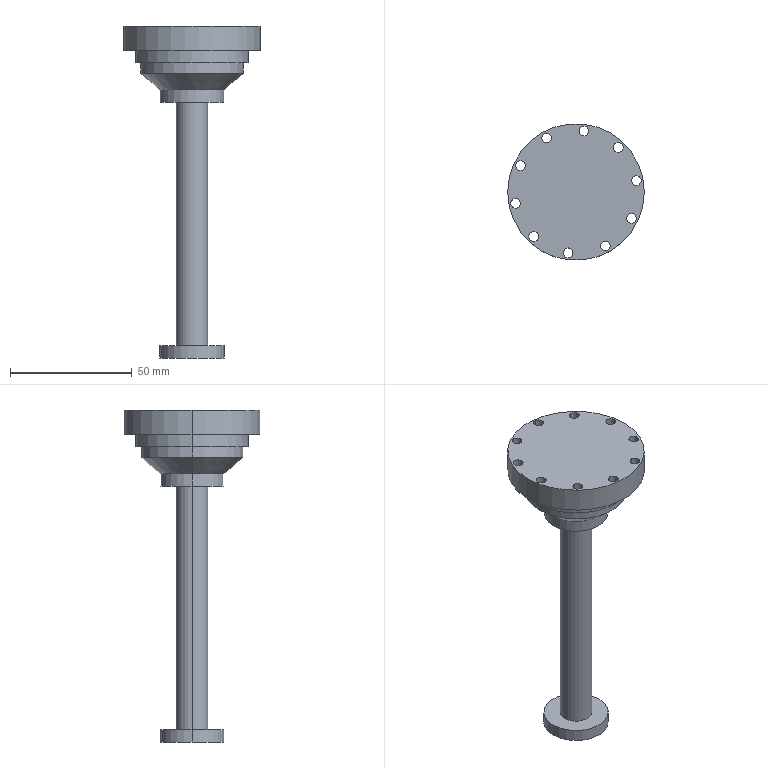Part | SolidWorks | features CirPattern 1, Cut 1, ICE 1, RevCut 1, Revolution 1 | 1 solid | 40 faces | box 56 x 56 x 136.215 mm | volume 62854 mm3 | cylinder 26 | cone 8 | plane 6 | commonest cylinder face diameters 4 x20 13.058 x2 42 x2 56 x2
STEP:
#1=CARTESIAN_POINT('',(-0.7415,66.642,15.));
#2=VERTEX_POINT('',#1);
#3=CARTESIAN_POINT('',(-4.741,66.642,15.));
#4=VERTEX_POINT('',#3);
#5=CARTESIAN_POINT('',(-2.741,66.642,15.));
#6=DIRECTION('',(0.,0.,-1.));
#7=DIRECTION('',(-0.809,0.5878,0.));
#8=AXIS2_PLACEMENT_3D('',#5,#6,#7);
#9=CIRCLE('',#8,2.);
#10=EDGE_CURVE('',#2,#4,#9,.T.);
#11=ORIENTED_EDGE('',*,*,#10,.F.);
#12=CARTESIAN_POINT('',(-0.7415,66.642,5.));
#13=VERTEX_POINT('',#12);
#14=CARTESIAN_POINT('',(-0.7415,66.642,15.));
#15=DIRECTION('',(0.,0.,-1.));
#16=VECTOR('',#15,1000.);
#17=LINE('',#14,#16);
#18=EDGE_CURVE('',#2,#13,#17,.T.);
#19=ORIENTED_EDGE('',*,*,#18,.T.);
#20=CARTESIAN_POINT('',(-4.741,66.642,5.));
#21=VERTEX_POINT('',#20);
#22=CARTESIAN_POINT('',(-2.741,66.642,5.));
#23=DIRECTION('',(0.,0.,-1.));
#24=DIRECTION('',(-0.809,0.5878,0.));
#25=AXIS2_PLACEMENT_3D('',#22,#23,#24);
#26=CIRCLE('',#25,2.);
#27=EDGE_CURVE('',#13,#21,#26,.T.);
#28=ORIENTED_EDGE('',*,*,#27,.T.);
#29=CARTESIAN_POINT('',(-4.741,66.642,15.));
#30=DIRECTION('',(0.,0.,-1.));
#31=VECTOR('',#30,1000.);
#32=LINE('',#29,#31);
#33=EDGE_CURVE('',#4,#21,#32,.T.);
#34=ORIENTED_EDGE('',*,*,#33,.F.);
#35=EDGE_LOOP('',(#11,#19,#28,#34));
#36=FACE_OUTER_BOUND('',#35,.T.);
#37=CARTESIAN_POINT('',(-2.741,66.642,15.));
#38=DIRECTION('',(0.,0.,-1.));
#39=DIRECTION('',(-1.,0.,0.));
#40=AXIS2_PLACEMENT_3D('',#37,#38,#39);
#41=CYLINDRICAL_SURFACE('',#40,2.);
#42=ADVANCED_FACE('',(#36),#41,.F.);
#43=CARTESIAN_POINT('',(7.956,75.944,15.));
#44=VERTEX_POINT('',#43);
#45=CARTESIAN_POINT('',(7.956,79.944,15.));
#46=VERTEX_POINT('',#45);
#47=CARTESIAN_POINT('',(7.956,77.944,15.));
#48=DIRECTION('',(0.,0.,-1.));
#49=DIRECTION('',(-0.309,0.9511,0.));
#50=AXIS2_PLACEMENT_3D('',#47,#48,#49);
#51=CIRCLE('',#50,2.);
#52=EDGE_CURVE('',#44,#46,#51,.T.);
#53=ORIENTED_EDGE('',*,*,#52,.F.);
#54=CARTESIAN_POINT('',(7.956,75.944,5.));
#55=VERTEX_POINT('',#54);
#56=CARTESIAN_POINT('',(7.956,75.944,15.));
#57=DIRECTION('',(0.,0.,-1.));
#58=VECTOR('',#57,1000.);
#59=LINE('',#56,#58);
#60=EDGE_CURVE('',#44,#55,#59,.T.);
#61=ORIENTED_EDGE('',*,*,#60,.T.);
#62=CARTESIAN_POINT('',(7.956,79.944,5.));
#63=VERTEX_POINT('',#62);
#64=CARTESIAN_POINT('',(7.956,77.944,5.));
#65=DIRECTION('',(0.,0.,-1.));
#66=DIRECTION('',(-0.309,0.9511,0.));
#67=AXIS2_PLACEMENT_3D('',#64,#65,#66);
#68=CIRCLE('',#67,2.);
#69=EDGE_CURVE('',#55,#63,#68,.T.);
#70=ORIENTED_EDGE('',*,*,#69,.T.);
#71=CARTESIAN_POINT('',(7.956,79.944,15.));
#72=DIRECTION('',(0.,0.,-1.));
#73=VECTOR('',#72,1000.);
#74=LINE('',#71,#73);
#75=EDGE_CURVE('',#46,#63,#74,.T.);
#76=ORIENTED_EDGE('',*,*,#75,.F.);
#77=EDGE_LOOP('',(#53,#61,#70,#76));
#78=FACE_OUTER_BOUND('',#77,.T.);
#79=CARTESIAN_POINT('',(7.956,77.944,15.));
#80=DIRECTION('',(0.,0.,-1.));
#81=DIRECTION('',(0.,1.,0.));
#82=AXIS2_PLACEMENT_3D('',#79,#80,#81);
#83=CYLINDRICAL_SURFACE('',#82,2.);
#84=ADVANCED_FACE('',(#78),#83,.F.);
#85=CARTESIAN_POINT('',(23.255,78.8,15.));
#86=VERTEX_POINT('',#85);
#87=CARTESIAN_POINT('',(23.255,82.8,15.));
#88=VERTEX_POINT('',#87);
#89=CARTESIAN_POINT('',(23.255,80.8,15.));
#90=DIRECTION('',(0.,0.,-1.));
#91=DIRECTION('',(0.309,0.9511,0.));
#92=AXIS2_PLACEMENT_3D('',#89,#90,#91);
#93=CIRCLE('',#92,2.);
#94=EDGE_CURVE('',#86,#88,#93,.T.);
#95=ORIENTED_EDGE('',*,*,#94,.F.);
#96=CARTESIAN_POINT('',(23.255,78.8,5.));
#97=VERTEX_POINT('',#96);
#98=CARTESIAN_POINT('',(23.255,78.8,15.));
#99=DIRECTION('',(0.,0.,-1.));
#100=VECTOR('',#99,1000.);
#101=LINE('',#98,#100);
#102=EDGE_CURVE('',#86,#97,#101,.T.);
#103=ORIENTED_EDGE('',*,*,#102,.T.);
#104=CARTESIAN_POINT('',(23.255,82.8,5.));
#105=VERTEX_POINT('',#104);
#106=CARTESIAN_POINT('',(23.255,80.8,5.));
#107=DIRECTION('',(0.,0.,-1.));
#108=DIRECTION('',(0.309,0.9511,0.));
#109=AXIS2_PLACEMENT_3D('',#106,#107,#108);
#110=CIRCLE('',#109,2.);
#111=EDGE_CURVE('',#97,#105,#110,.T.);
#112=ORIENTED_EDGE('',*,*,#111,.T.);
#113=CARTESIAN_POINT('',(23.255,82.8,15.));
#114=DIRECTION('',(0.,0.,-1.));
#115=VECTOR('',#114,1000.);
#116=LINE('',#113,#115);
#117=EDGE_CURVE('',#88,#105,#116,.T.);
#118=ORIENTED_EDGE('',*,*,#117,.F.);
#119=EDGE_LOOP('',(#95,#103,#112,#118));
#120=FACE_OUTER_BOUND('',#119,.T.);
#121=CARTESIAN_POINT('',(23.255,80.8,15.));
#122=DIRECTION('',(0.,0.,-1.));
#123=DIRECTION('',(0.,1.,0.));
#124=AXIS2_PLACEMENT_3D('',#121,#122,#123);
#125=CYLINDRICAL_SURFACE('',#124,2.);
#126=ADVANCED_FACE('',(#120),#125,.F.);
#127=CARTESIAN_POINT('',(37.31,72.118,15.));
#128=VERTEX_POINT('',#127);
#129=CARTESIAN_POINT('',(37.31,76.118,15.));
#130=VERTEX_POINT('',#129);
#131=CARTESIAN_POINT('',(37.31,74.118,15.));
#132=DIRECTION('',(0.,0.,-1.));
#133=DIRECTION('',(0.809,0.5878,0.));
#134=AXIS2_PLACEMENT_3D('',#131,#132,#133);
#135=CIRCLE('',#134,2.);
#136=EDGE_CURVE('',#128,#130,#135,.T.);
#137=ORIENTED_EDGE('',*,*,#136,.F.);
#138=CARTESIAN_POINT('',(37.31,72.118,5.));
#139=VERTEX_POINT('',#138);
#140=CARTESIAN_POINT('',(37.31,72.118,15.));
#141=DIRECTION('',(0.,0.,-1.));
#142=VECTOR('',#141,1000.);
#143=LINE('',#140,#142);
#144=EDGE_CURVE('',#128,#139,#143,.T.);
#145=ORIENTED_EDGE('',*,*,#144,.T.);
#146=CARTESIAN_POINT('',(37.31,76.118,5.));
#147=VERTEX_POINT('',#146);
#148=CARTESIAN_POINT('',(37.31,74.118,5.));
#149=DIRECTION('',(0.,0.,-1.));
#150=DIRECTION('',(0.809,0.5878,0.));
#151=AXIS2_PLACEMENT_3D('',#148,#149,#150);
#152=CIRCLE('',#151,2.);
#153=EDGE_CURVE('',#139,#147,#152,.T.);
#154=ORIENTED_EDGE('',*,*,#153,.T.);
#155=CARTESIAN_POINT('',(37.31,76.118,15.));
#156=DIRECTION('',(0.,0.,-1.));
#157=VECTOR('',#156,1000.);
#158=LINE('',#155,#157);
#159=EDGE_CURVE('',#130,#147,#158,.T.);
#160=ORIENTED_EDGE('',*,*,#159,.F.);
#161=EDGE_LOOP('',(#137,#145,#154,#160));
#162=FACE_OUTER_BOUND('',#161,.T.);
#163=CARTESIAN_POINT('',(37.31,74.118,15.));
#164=DIRECTION('',(0.,0.,-1.));
#165=DIRECTION('',(0.,1.,0.));
#166=AXIS2_PLACEMENT_3D('',#163,#164,#165);
#167=CYLINDRICAL_SURFACE('',#166,2.);
#168=ADVANCED_FACE('',(#162),#167,.F.);
#169=CARTESIAN_POINT('',(46.753,60.451,15.));
#170=VERTEX_POINT('',#169);
#171=CARTESIAN_POINT('',(42.753,60.451,15.));
#172=VERTEX_POINT('',#171);
#173=CARTESIAN_POINT('',(44.753,60.451,15.));
#174=DIRECTION('',(0.,0.,-1.));
#175=DIRECTION('',(1.,0.,0.));
#176=AXIS2_PLACEMENT_3D('',#173,#174,#175);
#177=CIRCLE('',#176,2.);
#178=EDGE_CURVE('',#170,#172,#177,.T.);
#179=ORIENTED_EDGE('',*,*,#178,.F.);
#180=CARTESIAN_POINT('',(46.753,60.451,5.));
#181=VERTEX_POINT('',#180);
#182=CARTESIAN_POINT('',(46.753,60.451,15.));
#183=DIRECTION('',(0.,0.,-1.));
#184=VECTOR('',#183,1000.);
#185=LINE('',#182,#184);
#186=EDGE_CURVE('',#170,#181,#185,.T.);
#187=ORIENTED_EDGE('',*,*,#186,.T.);
#188=CARTESIAN_POINT('',(42.753,60.451,5.));
#189=VERTEX_POINT('',#188);
#190=CARTESIAN_POINT('',(44.753,60.451,5.));
#191=DIRECTION('',(0.,0.,-1.));
#192=DIRECTION('',(1.,0.,0.));
#193=AXIS2_PLACEMENT_3D('',#190,#191,#192);
#194=CIRCLE('',#193,2.);
#195=EDGE_CURVE('',#181,#189,#194,.T.);
#196=ORIENTED_EDGE('',*,*,#195,.T.);
#197=CARTESIAN_POINT('',(42.753,60.451,15.));
#198=DIRECTION('',(0.,0.,-1.));
#199=VECTOR('',#198,1000.);
#200=LINE('',#197,#199);
#201=EDGE_CURVE('',#172,#189,#200,.T.);
#202=ORIENTED_EDGE('',*,*,#201,.F.);
#203=EDGE_LOOP('',(#179,#187,#196,#202));
#204=FACE_OUTER_BOUND('',#203,.T.);
#205=CARTESIAN_POINT('',(44.753,60.451,15.));
#206=DIRECTION('',(0.,0.,-1.));
#207=DIRECTION('',(-1.,0.,0.));
#208=AXIS2_PLACEMENT_3D('',#205,#206,#207);
#209=CYLINDRICAL_SURFACE('',#208,2.);
#210=ADVANCED_FACE('',(#204),#209,.F.);
#211=CARTESIAN_POINT('',(44.741,45.019,15.));
#212=VERTEX_POINT('',#211);
#213=CARTESIAN_POINT('',(40.741,45.019,15.));
#214=VERTEX_POINT('',#213);
#215=CARTESIAN_POINT('',(42.741,45.019,15.));
#216=DIRECTION('',(0.,0.,-1.));
#217=DIRECTION('',(0.809,-0.5878,0.));
#218=AXIS2_PLACEMENT_3D('',#215,#216,#217);
#219=CIRCLE('',#218,2.);
#220=EDGE_CURVE('',#212,#214,#219,.T.);
#221=ORIENTED_EDGE('',*,*,#220,.F.);
#222=CARTESIAN_POINT('',(44.741,45.019,5.));
#223=VERTEX_POINT('',#222);
#224=CARTESIAN_POINT('',(44.741,45.019,15.));
#225=DIRECTION('',(0.,0.,-1.));
#226=VECTOR('',#225,1000.);
#227=LINE('',#224,#226);
#228=EDGE_CURVE('',#212,#223,#227,.T.);
#229=ORIENTED_EDGE('',*,*,#228,.T.);
#230=CARTESIAN_POINT('',(40.741,45.019,5.));
#231=VERTEX_POINT('',#230);
#232=CARTESIAN_POINT('',(42.741,45.019,5.));
#233=DIRECTION('',(0.,0.,-1.));
#234=DIRECTION('',(0.809,-0.5878,0.));
#235=AXIS2_PLACEMENT_3D('',#232,#233,#234);
#236=CIRCLE('',#235,2.);
#237=EDGE_CURVE('',#223,#231,#236,.T.);
#238=ORIENTED_EDGE('',*,*,#237,.T.);
#239=CARTESIAN_POINT('',(40.741,45.019,15.));
#240=DIRECTION('',(0.,0.,-1.));
#241=VECTOR('',#240,1000.);
#242=LINE('',#239,#241);
#243=EDGE_CURVE('',#214,#231,#242,.T.);
#244=ORIENTED_EDGE('',*,*,#243,.F.);
#245=EDGE_LOOP('',(#221,#229,#238,#244));
#246=FACE_OUTER_BOUND('',#245,.T.);
#247=CARTESIAN_POINT('',(42.741,45.019,15.));
#248=DIRECTION('',(0.,0.,-1.));
#249=DIRECTION('',(-1.,0.,0.));
#250=AXIS2_PLACEMENT_3D('',#247,#248,#249);
#251=CYLINDRICAL_SURFACE('',#250,2.);
#252=ADVANCED_FACE('',(#246),#251,.F.);
#253=CARTESIAN_POINT('',(32.044,31.717,15.));
#254=VERTEX_POINT('',#253);
#255=CARTESIAN_POINT('',(32.044,35.717,15.));
#256=VERTEX_POINT('',#255);
#257=CARTESIAN_POINT('',(32.044,33.717,15.));
#258=DIRECTION('',(0.,0.,-1.));
#259=DIRECTION('',(0.309,-0.9511,0.));
#260=AXIS2_PLACEMENT_3D('',#257,#258,#259);
#261=CIRCLE('',#260,2.);
#262=EDGE_CURVE('',#254,#256,#261,.T.);
#263=ORIENTED_EDGE('',*,*,#262,.F.);
#264=CARTESIAN_POINT('',(32.044,31.717,5.));
#265=VERTEX_POINT('',#264);
#266=CARTESIAN_POINT('',(32.044,31.717,15.));
#267=DIRECTION('',(0.,0.,-1.));
#268=VECTOR('',#267,1000.);
#269=LINE('',#266,#268);
#270=EDGE_CURVE('',#254,#265,#269,.T.);
#271=ORIENTED_EDGE('',*,*,#270,.T.);
#272=CARTESIAN_POINT('',(32.044,35.717,5.));
#273=VERTEX_POINT('',#272);
#274=CARTESIAN_POINT('',(32.044,33.717,5.));
#275=DIRECTION('',(0.,0.,-1.));
#276=DIRECTION('',(0.309,-0.9511,0.));
#277=AXIS2_PLACEMENT_3D('',#274,#275,#276);
#278=CIRCLE('',#277,2.);
#279=EDGE_CURVE('',#265,#273,#278,.T.);
#280=ORIENTED_EDGE('',*,*,#279,.T.);
#281=CARTESIAN_POINT('',(32.044,35.717,15.));
#282=DIRECTION('',(0.,0.,-1.));
#283=VECTOR('',#282,1000.);
#284=LINE('',#281,#283);
#285=EDGE_CURVE('',#256,#273,#284,.T.);
#286=ORIENTED_EDGE('',*,*,#285,.F.);
#287=EDGE_LOOP('',(#263,#271,#280,#286));
#288=FACE_OUTER_BOUND('',#287,.T.);
#289=CARTESIAN_POINT('',(32.044,33.717,15.));
#290=DIRECTION('',(0.,0.,-1.));
#291=DIRECTION('',(0.,1.,0.));
#292=AXIS2_PLACEMENT_3D('',#289,#290,#291);
#293=CYLINDRICAL_SURFACE('',#292,2.);
#294=ADVANCED_FACE('',(#288),#293,.F.);
#295=CARTESIAN_POINT('',(16.745,28.861,15.));
#296=VERTEX_POINT('',#295);
#297=CARTESIAN_POINT('',(16.745,32.861,15.));
#298=VERTEX_POINT('',#297);
#299=CARTESIAN_POINT('',(16.745,30.861,15.));
#300=DIRECTION('',(0.,0.,-1.));
#301=DIRECTION('',(-0.309,-0.9511,0.));
#302=AXIS2_PLACEMENT_3D('',#299,#300,#301);
#303=CIRCLE('',#302,2.);
#304=EDGE_CURVE('',#296,#298,#303,.T.);
#305=ORIENTED_EDGE('',*,*,#304,.F.);
#306=CARTESIAN_POINT('',(16.745,28.861,5.));
#307=VERTEX_POINT('',#306);
#308=CARTESIAN_POINT('',(16.745,28.861,15.));
#309=DIRECTION('',(0.,0.,-1.));
#310=VECTOR('',#309,1000.);
#311=LINE('',#308,#310);
#312=EDGE_CURVE('',#296,#307,#311,.T.);
#313=ORIENTED_EDGE('',*,*,#312,.T.);
#314=CARTESIAN_POINT('',(16.745,32.861,5.));
#315=VERTEX_POINT('',#314);
#316=CARTESIAN_POINT('',(16.745,30.861,5.));
#317=DIRECTION('',(0.,0.,-1.));
#318=DIRECTION('',(-0.309,-0.9511,0.));
#319=AXIS2_PLACEMENT_3D('',#316,#317,#318);
#320=CIRCLE('',#319,2.);
#321=EDGE_CURVE('',#307,#315,#320,.T.);
#322=ORIENTED_EDGE('',*,*,#321,.T.);
#323=CARTESIAN_POINT('',(16.745,32.861,15.));
#324=DIRECTION('',(0.,0.,-1.));
#325=VECTOR('',#324,1000.);
#326=LINE('',#323,#325);
#327=EDGE_CURVE('',#298,#315,#326,.T.);
#328=ORIENTED_EDGE('',*,*,#327,.F.);
#329=EDGE_LOOP('',(#305,#313,#322,#328));
#330=FACE_OUTER_BOUND('',#329,.T.);
#331=CARTESIAN_POINT('',(16.745,30.861,15.));
#332=DIRECTION('',(0.,0.,-1.));
#333=DIRECTION('',(0.,1.,0.));
#334=AXIS2_PLACEMENT_3D('',#331,#332,#333);
#335=CYLINDRICAL_SURFACE('',#334,2.);
#336=ADVANCED_FACE('',(#330),#335,.F.);
#337=CARTESIAN_POINT('',(2.69,35.543,15.));
#338=VERTEX_POINT('',#337);
#339=CARTESIAN_POINT('',(2.69,39.543,15.));
#340=VERTEX_POINT('',#339);
#341=CARTESIAN_POINT('',(2.69,37.543,15.));
#342=DIRECTION('',(0.,0.,-1.));
#343=DIRECTION('',(-0.809,-0.5878,0.));
#344=AXIS2_PLACEMENT_3D('',#341,#342,#343);
#345=CIRCLE('',#344,2.);
#346=EDGE_CURVE('',#338,#340,#345,.T.);
#347=ORIENTED_EDGE('',*,*,#346,.F.);
#348=CARTESIAN_POINT('',(2.69,35.543,5.));
#349=VERTEX_POINT('',#348);
#350=CARTESIAN_POINT('',(2.69,35.543,15.));
#351=DIRECTION('',(0.,0.,-1.));
#352=VECTOR('',#351,1000.);
#353=LINE('',#350,#352);
#354=EDGE_CURVE('',#338,#349,#353,.T.);
#355=ORIENTED_EDGE('',*,*,#354,.T.);
#356=CARTESIAN_POINT('',(2.69,39.543,5.));
#357=VERTEX_POINT('',#356);
#358=CARTESIAN_POINT('',(2.69,37.543,5.));
#359=DIRECTION('',(0.,0.,-1.));
#360=DIRECTION('',(-0.809,-0.5878,0.));
#361=AXIS2_PLACEMENT_3D('',#358,#359,#360);
#362=CIRCLE('',#361,2.);
#363=EDGE_CURVE('',#349,#357,#362,.T.);
#364=ORIENTED_EDGE('',*,*,#363,.T.);
#365=CARTESIAN_POINT('',(2.69,39.543,15.));
#366=DIRECTION('',(0.,0.,-1.));
#367=VECTOR('',#366,1000.);
#368=LINE('',#365,#367);
#369=EDGE_CURVE('',#340,#357,#368,.T.);
#370=ORIENTED_EDGE('',*,*,#369,.F.);
#371=EDGE_LOOP('',(#347,#355,#364,#370));
#372=FACE_OUTER_BOUND('',#371,.T.);
#373=CARTESIAN_POINT('',(2.69,37.543,15.));
#374=DIRECTION('',(0.,0.,-1.));
#375=DIRECTION('',(0.,1.,0.));
#376=AXIS2_PLACEMENT_3D('',#373,#374,#375);
#377=CYLINDRICAL_SURFACE('',#376,2.);
#378=ADVANCED_FACE('',(#372),#377,.F.);
#379=CARTESIAN_POINT('',(-2.753,51.21,15.));
#380=VERTEX_POINT('',#379);
#381=CARTESIAN_POINT('',(-6.753,51.21,15.));
#382=VERTEX_POINT('',#381);
#383=CARTESIAN_POINT('',(-4.753,51.21,15.));
#384=DIRECTION('',(0.,0.,-1.));
#385=DIRECTION('',(-1.,0.,0.));
#386=AXIS2_PLACEMENT_3D('',#383,#384,#385);
#387=CIRCLE('',#386,2.);
#388=EDGE_CURVE('',#380,#382,#387,.T.);
#389=ORIENTED_EDGE('',*,*,#388,.F.);
#390=CARTESIAN_POINT('',(-2.753,51.21,5.));
#391=VERTEX_POINT('',#390);
#392=CARTESIAN_POINT('',(-2.753,51.21,15.));
#393=DIRECTION('',(0.,0.,-1.));
#394=VECTOR('',#393,1000.);
#395=LINE('',#392,#394);
#396=EDGE_CURVE('',#380,#391,#395,.T.);
#397=ORIENTED_EDGE('',*,*,#396,.T.);
#398=CARTESIAN_POINT('',(-6.753,51.21,5.));
#399=VERTEX_POINT('',#398);
#400=CARTESIAN_POINT('',(-4.753,51.21,5.));
#401=DIRECTION('',(0.,0.,-1.));
#402=DIRECTION('',(-1.,0.,0.));
#403=AXIS2_PLACEMENT_3D('',#400,#401,#402);
#404=CIRCLE('',#403,2.);
#405=EDGE_CURVE('',#391,#399,#404,.T.);
#406=ORIENTED_EDGE('',*,*,#405,.T.);
#407=CARTESIAN_POINT('',(-6.753,51.21,15.));
#408=DIRECTION('',(0.,0.,-1.));
#409=VECTOR('',#408,1000.);
#410=LINE('',#407,#409);
#411=EDGE_CURVE('',#382,#399,#410,.T.);
#412=ORIENTED_EDGE('',*,*,#411,.F.);
#413=EDGE_LOOP('',(#389,#397,#406,#412));
#414=FACE_OUTER_BOUND('',#413,.T.);
#415=CARTESIAN_POINT('',(-4.753,51.21,15.));
#416=DIRECTION('',(0.,0.,-1.));
#417=DIRECTION('',(-1.,0.,0.));
#418=AXIS2_PLACEMENT_3D('',#415,#416,#417);
#419=CYLINDRICAL_SURFACE('',#418,2.);
#420=ADVANCED_FACE('',(#414),#419,.F.);
#421=CARTESIAN_POINT('',(-8.,55.831,5.));
#422=VERTEX_POINT('',#421);
#423=CARTESIAN_POINT('',(48.,55.831,5.));
#424=VERTEX_POINT('',#423);
#425=CARTESIAN_POINT('',(20.,55.831,5.));
#426=DIRECTION('',(0.,0.,-1.));
#427=DIRECTION('',(-1.,0.,0.));
#428=AXIS2_PLACEMENT_3D('',#425,#426,#427);
#429=CIRCLE('',#428,28.);
#430=EDGE_CURVE('',#422,#424,#429,.T.);
#431=ORIENTED_EDGE('',*,*,#430,.F.);
#432=CARTESIAN_POINT('',(-8.,55.831,15.));
#433=VERTEX_POINT('',#432);
#434=CARTESIAN_POINT('',(-8.,55.831,5.));
#435=DIRECTION('',(0.,0.,1.));
#436=VECTOR('',#435,1000.);
#437=LINE('',#434,#436);
#438=EDGE_CURVE('',#422,#433,#437,.T.);
#439=ORIENTED_EDGE('',*,*,#438,.T.);
#440=CARTESIAN_POINT('',(48.,55.831,15.));
#441=VERTEX_POINT('',#440);
#442=CARTESIAN_POINT('',(20.,55.831,15.));
#443=DIRECTION('',(0.,0.,-1.));
#444=DIRECTION('',(-1.,0.,0.));
#445=AXIS2_PLACEMENT_3D('',#442,#443,#444);
#446=CIRCLE('',#445,28.);
#447=EDGE_CURVE('',#433,#441,#446,.T.);
#448=ORIENTED_EDGE('',*,*,#447,.T.);
#449=CARTESIAN_POINT('',(48.,55.831,5.));
#450=DIRECTION('',(0.,0.,1.));
#451=VECTOR('',#450,1000.);
#452=LINE('',#449,#451);
#453=EDGE_CURVE('',#424,#441,#452,.T.);
#454=ORIENTED_EDGE('',*,*,#453,.F.);
#455=EDGE_LOOP('',(#431,#439,#448,#454));
#456=FACE_OUTER_BOUND('',#455,.T.);
#457=CARTESIAN_POINT('',(20.,55.831,5.));
#458=DIRECTION('',(0.,0.,1.));
#459=DIRECTION('',(1.,0.,0.));
#460=AXIS2_PLACEMENT_3D('',#457,#458,#459);
#461=CYLINDRICAL_SURFACE('',#460,28.);
#462=ADVANCED_FACE('',(#456),#461,.T.);
#463=CARTESIAN_POINT('',(6.805,55.831,-116.215));
#464=VERTEX_POINT('',#463);
#465=CARTESIAN_POINT('',(33.195,55.831,-116.215));
#466=VERTEX_POINT('',#465);
#467=CARTESIAN_POINT('',(20.,55.831,-116.215));
#468=DIRECTION('',(0.,0.,-1.));
#469=DIRECTION('',(1.,0.,0.));
#470=AXIS2_PLACEMENT_3D('',#467,#468,#469);
#471=CIRCLE('',#470,13.195);
#472=EDGE_CURVE('',#464,#466,#471,.T.);
#473=ORIENTED_EDGE('',*,*,#472,.T.);
#474=CARTESIAN_POINT('',(33.204,55.831,-121.215));
#475=VERTEX_POINT('',#474);
#476=CARTESIAN_POINT('',(33.,55.831,-11.215));
#477=DIRECTION('',(0.001855,0.,-1.));
#478=VECTOR('',#477,1000.);
#479=LINE('',#476,#478);
#480=EDGE_CURVE('',#466,#475,#479,.T.);
#481=ORIENTED_EDGE('',*,*,#480,.T.);
#482=CARTESIAN_POINT('',(6.796,55.831,-121.215));
#483=VERTEX_POINT('',#482);
#484=CARTESIAN_POINT('',(20.,55.831,-121.215));
#485=DIRECTION('',(0.,0.,1.));
#486=DIRECTION('',(1.,0.,0.));
#487=AXIS2_PLACEMENT_3D('',#484,#485,#486);
#488=CIRCLE('',#487,13.204);
#489=EDGE_CURVE('',#475,#483,#488,.T.);
#490=ORIENTED_EDGE('',*,*,#489,.T.);
#491=CARTESIAN_POINT('',(7.,55.831,-11.215));
#492=DIRECTION('',(-0.001855,0.,-1.));
#493=VECTOR('',#492,1000.);
#494=LINE('',#491,#493);
#495=EDGE_CURVE('',#464,#483,#494,.T.);
#496=ORIENTED_EDGE('',*,*,#495,.F.);
#497=EDGE_LOOP('',(#473,#481,#490,#496));
#498=FACE_OUTER_BOUND('',#497,.T.);
#499=CARTESIAN_POINT('',(20.,55.831,-11.215));
#500=DIRECTION('',(0.,0.,-1.));
#501=DIRECTION('',(-1.,0.,0.));
#502=AXIS2_PLACEMENT_3D('',#499,#500,#501);
#503=CONICAL_SURFACE('',#502,13.,0.001855);
#504=ADVANCED_FACE('',(#498),#503,.T.);
#505=CARTESIAN_POINT('',(26.529,55.831,-116.215));
#506=VERTEX_POINT('',#505);
#507=CARTESIAN_POINT('',(13.471,55.831,-116.215));
#508=VERTEX_POINT('',#507);
#509=CARTESIAN_POINT('',(20.,55.831,-116.215));
#510=DIRECTION('',(0.,0.,1.));
#511=DIRECTION('',(1.,0.,0.));
#512=AXIS2_PLACEMENT_3D('',#509,#510,#511);
#513=CIRCLE('',#512,6.529);
#514=EDGE_CURVE('',#506,#508,#513,.T.);
#515=ORIENTED_EDGE('',*,*,#514,.T.);
#516=CARTESIAN_POINT('',(13.471,55.831,-16.215));
#517=VERTEX_POINT('',#516);
#518=CARTESIAN_POINT('',(13.471,55.831,-11.215));
#519=DIRECTION('',(0.,0.,1.));
#520=VECTOR('',#519,1000.);
#521=LINE('',#518,#520);
#522=EDGE_CURVE('',#508,#517,#521,.T.);
#523=ORIENTED_EDGE('',*,*,#522,.T.);
#524=CARTESIAN_POINT('',(26.529,55.831,-16.215));
#525=VERTEX_POINT('',#524);
#526=CARTESIAN_POINT('',(20.,55.831,-16.215));
#527=DIRECTION('',(0.,0.,1.));
#528=DIRECTION('',(1.,0.,0.));
#529=AXIS2_PLACEMENT_3D('',#526,#527,#528);
#530=CIRCLE('',#529,6.529);
#531=EDGE_CURVE('',#525,#517,#530,.T.);
#532=ORIENTED_EDGE('',*,*,#531,.F.);
#533=CARTESIAN_POINT('',(26.529,55.831,-11.215));
#534=DIRECTION('',(0.,0.,1.));
#535=VECTOR('',#534,1000.);
#536=LINE('',#533,#535);
#537=EDGE_CURVE('',#506,#525,#536,.T.);
#538=ORIENTED_EDGE('',*,*,#537,.F.);
#539=EDGE_LOOP('',(#515,#523,#532,#538));
#540=FACE_OUTER_BOUND('',#539,.T.);
#541=CARTESIAN_POINT('',(20.,55.831,-11.215));
#542=DIRECTION('',(0.,0.,1.));
#543=DIRECTION('',(1.,0.,0.));
#544=AXIS2_PLACEMENT_3D('',#541,#542,#543);
#545=CYLINDRICAL_SURFACE('',#544,6.529);
#546=ADVANCED_FACE('',(#540),#545,.T.);
#547=CARTESIAN_POINT('',(42.991,55.831,5.));
#548=VERTEX_POINT('',#547);
#549=CARTESIAN_POINT('',(-2.991,55.831,5.));
#550=VERTEX_POINT('',#549);
#551=CARTESIAN_POINT('',(20.,55.831,5.));
#552=DIRECTION('',(0.,0.,1.));
#553=DIRECTION('',(-1.,0.,0.));
#554=AXIS2_PLACEMENT_3D('',#551,#552,#553);
#555=CIRCLE('',#554,22.991);
#556=EDGE_CURVE('',#548,#550,#555,.T.);
#557=ORIENTED_EDGE('',*,*,#556,.F.);
#558=CARTESIAN_POINT('',(43.,55.831,0.));
#559=VERTEX_POINT('',#558);
#560=CARTESIAN_POINT('',(42.972,55.831,15.));
#561=DIRECTION('',(0.001855,0.,-1.));
#562=VECTOR('',#561,1000.);
#563=LINE('',#560,#562);
#564=EDGE_CURVE('',#548,#559,#563,.T.);
#565=ORIENTED_EDGE('',*,*,#564,.T.);
#566=CARTESIAN_POINT('',(-3.,55.831,0.));
#567=VERTEX_POINT('',#566);
#568=CARTESIAN_POINT('',(20.,55.831,0.));
#569=DIRECTION('',(0.,0.,1.));
#570=DIRECTION('',(1.,0.,0.));
#571=AXIS2_PLACEMENT_3D('',#568,#569,#570);
#572=CIRCLE('',#571,23.);
#573=EDGE_CURVE('',#559,#567,#572,.T.);
#574=ORIENTED_EDGE('',*,*,#573,.T.);
#575=CARTESIAN_POINT('',(-2.972,55.831,15.));
#576=DIRECTION('',(-0.001855,0.,-1.));
#577=VECTOR('',#576,1000.);
#578=LINE('',#575,#577);
#579=EDGE_CURVE('',#550,#567,#578,.T.);
#580=ORIENTED_EDGE('',*,*,#579,.F.);
#581=EDGE_LOOP('',(#557,#565,#574,#580));
#582=FACE_OUTER_BOUND('',#581,.T.);
#583=CARTESIAN_POINT('',(20.,55.831,15.));
#584=DIRECTION('',(0.,0.,-1.));
#585=DIRECTION('',(-1.,0.,0.));
#586=AXIS2_PLACEMENT_3D('',#583,#584,#585);
#587=CONICAL_SURFACE('',#586,22.972,0.001855);
#588=ADVANCED_FACE('',(#582),#587,.T.);
#589=CARTESIAN_POINT('',(33.,55.831,-11.215));
#590=VERTEX_POINT('',#589);
#591=CARTESIAN_POINT('',(7.,55.831,-11.215));
#592=VERTEX_POINT('',#591);
#593=CARTESIAN_POINT('',(20.,55.831,-11.215));
#594=DIRECTION('',(0.,0.,1.));
#595=DIRECTION('',(1.,0.,0.));
#596=AXIS2_PLACEMENT_3D('',#593,#594,#595);
#597=CIRCLE('',#596,13.);
#598=EDGE_CURVE('',#590,#592,#597,.T.);
#599=ORIENTED_EDGE('',*,*,#598,.T.);
#600=CARTESIAN_POINT('',(-1.,55.831,-4.383));
#601=VERTEX_POINT('',#600);
#602=CARTESIAN_POINT('',(-1.,55.831,-4.383));
#603=DIRECTION('',(-0.7605,0.,0.6494));
#604=VECTOR('',#603,1000.);
#605=LINE('',#602,#604);
#606=EDGE_CURVE('',#592,#601,#605,.T.);
#607=ORIENTED_EDGE('',*,*,#606,.T.);
#608=CARTESIAN_POINT('',(41.,55.831,-4.383));
#609=VERTEX_POINT('',#608);
#610=CARTESIAN_POINT('',(20.,55.831,-4.383));
#611=DIRECTION('',(0.,0.,1.));
#612=DIRECTION('',(1.,0.,0.));
#613=AXIS2_PLACEMENT_3D('',#610,#611,#612);
#614=CIRCLE('',#613,21.);
#615=EDGE_CURVE('',#609,#601,#614,.T.);
#616=ORIENTED_EDGE('',*,*,#615,.F.);
#617=CARTESIAN_POINT('',(41.,55.831,-4.383));
#618=DIRECTION('',(0.7605,0.,0.6494));
#619=VECTOR('',#618,1000.);
#620=LINE('',#617,#619);
#621=EDGE_CURVE('',#590,#609,#620,.T.);
#622=ORIENTED_EDGE('',*,*,#621,.F.);
#623=EDGE_LOOP('',(#599,#607,#616,#622));
#624=FACE_OUTER_BOUND('',#623,.T.);
#625=CARTESIAN_POINT('',(20.,55.831,-4.383));
#626=DIRECTION('',(0.,0.,1.));
#627=DIRECTION('',(1.,0.,0.));
#628=AXIS2_PLACEMENT_3D('',#625,#626,#627);
#629=CONICAL_SURFACE('',#628,21.,0.864);
#630=ADVANCED_FACE('',(#624),#629,.T.);
#631=ORIENTED_EDGE('',*,*,#615,.T.);
#632=CARTESIAN_POINT('',(-1.,55.831,0.));
#633=VERTEX_POINT('',#632);
#634=CARTESIAN_POINT('',(-1.,55.831,15.));
#635=DIRECTION('',(0.,0.,1.));
#636=VECTOR('',#635,1000.);
#637=LINE('',#634,#636);
#638=EDGE_CURVE('',#601,#633,#637,.T.);
#639=ORIENTED_EDGE('',*,*,#638,.T.);
#640=CARTESIAN_POINT('',(41.,55.831,0.));
#641=VERTEX_POINT('',#640);
#642=CARTESIAN_POINT('',(20.,55.831,0.));
#643=DIRECTION('',(0.,0.,1.));
#644=DIRECTION('',(1.,0.,0.));
#645=AXIS2_PLACEMENT_3D('',#642,#643,#644);
#646=CIRCLE('',#645,21.);
#647=EDGE_CURVE('',#641,#633,#646,.T.);
#648=ORIENTED_EDGE('',*,*,#647,.F.);
#649=CARTESIAN_POINT('',(41.,55.831,15.));
#650=DIRECTION('',(0.,0.,1.));
#651=VECTOR('',#650,1000.);
#652=LINE('',#649,#651);
#653=EDGE_CURVE('',#609,#641,#652,.T.);
#654=ORIENTED_EDGE('',*,*,#653,.F.);
#655=EDGE_LOOP('',(#631,#639,#648,#654));
#656=FACE_OUTER_BOUND('',#655,.T.);
#657=CARTESIAN_POINT('',(20.,55.831,15.));
#658=DIRECTION('',(0.,0.,1.));
#659=DIRECTION('',(1.,0.,0.));
#660=AXIS2_PLACEMENT_3D('',#657,#658,#659);
#661=CYLINDRICAL_SURFACE('',#660,21.);
#662=ADVANCED_FACE('',(#656),#661,.T.);
#663=ORIENTED_EDGE('',*,*,#598,.F.);
#664=CARTESIAN_POINT('',(33.009,55.831,-16.215));
#665=VERTEX_POINT('',#664);
#666=CARTESIAN_POINT('',(33.,55.831,-11.215));
#667=DIRECTION('',(0.001855,0.,-1.));
#668=VECTOR('',#667,1000.);
#669=LINE('',#666,#668);
#670=EDGE_CURVE('',#590,#665,#669,.T.);
#671=ORIENTED_EDGE('',*,*,#670,.T.);
#672=CARTESIAN_POINT('',(6.991,55.831,-16.215));
#673=VERTEX_POINT('',#672);
#674=CARTESIAN_POINT('',(20.,55.831,-16.215));
#675=DIRECTION('',(0.,0.,1.));
#676=DIRECTION('',(-1.,0.,0.));
#677=AXIS2_PLACEMENT_3D('',#674,#675,#676);
#678=CIRCLE('',#677,13.009);
#679=EDGE_CURVE('',#665,#673,#678,.T.);
#680=ORIENTED_EDGE('',*,*,#679,.T.);
#681=CARTESIAN_POINT('',(7.,55.831,-11.215));
#682=DIRECTION('',(-0.001855,0.,-1.));
#683=VECTOR('',#682,1000.);
#684=LINE('',#681,#683);
#685=EDGE_CURVE('',#592,#673,#684,.T.);
#686=ORIENTED_EDGE('',*,*,#685,.F.);
#687=EDGE_LOOP('',(#663,#671,#680,#686));
#688=FACE_OUTER_BOUND('',#687,.T.);
#689=CARTESIAN_POINT('',(20.,55.831,-11.215));
#690=DIRECTION('',(0.,0.,-1.));
#691=DIRECTION('',(-1.,0.,0.));
#692=AXIS2_PLACEMENT_3D('',#689,#690,#691);
#693=CONICAL_SURFACE('',#692,13.,0.001855);
#694=ADVANCED_FACE('',(#688),#693,.T.);
#695=ORIENTED_EDGE('',*,*,#670,.F.);
#696=CARTESIAN_POINT('',(20.,55.831,-11.215));
#697=DIRECTION('',(0.,0.,1.));
#698=DIRECTION('',(1.,0.,0.));
#699=AXIS2_PLACEMENT_3D('',#696,#697,#698);
#700=CIRCLE('',#699,13.);
#701=EDGE_CURVE('',#592,#590,#700,.T.);
#702=ORIENTED_EDGE('',*,*,#701,.F.);
#703=ORIENTED_EDGE('',*,*,#685,.T.);
#704=CARTESIAN_POINT('',(20.,55.831,-16.215));
#705=DIRECTION('',(0.,0.,1.));
#706=DIRECTION('',(-1.,0.,0.));
#707=AXIS2_PLACEMENT_3D('',#704,#705,#706);
#708=CIRCLE('',#707,13.009);
#709=EDGE_CURVE('',#673,#665,#708,.T.);
#710=ORIENTED_EDGE('',*,*,#709,.T.);
#711=EDGE_LOOP('',(#695,#702,#703,#710));
#712=FACE_OUTER_BOUND('',#711,.T.);
#713=CARTESIAN_POINT('',(20.,55.831,-11.215));
#714=DIRECTION('',(0.,0.,-1.));
#715=DIRECTION('',(-1.,0.,0.));
#716=AXIS2_PLACEMENT_3D('',#713,#714,#715);
#717=CONICAL_SURFACE('',#716,13.,0.001855);
#718=ADVANCED_FACE('',(#712),#717,.T.);
#719=ORIENTED_EDGE('',*,*,#647,.T.);
#720=CARTESIAN_POINT('',(20.,55.831,0.));
#721=DIRECTION('',(0.,0.,1.));
#722=DIRECTION('',(1.,0.,0.));
#723=AXIS2_PLACEMENT_3D('',#720,#721,#722);
#724=CIRCLE('',#723,21.);
#725=EDGE_CURVE('',#633,#641,#724,.T.);
#726=ORIENTED_EDGE('',*,*,#725,.T.);
#727=EDGE_LOOP('',(#719,#726));
#728=FACE_BOUND('',#727,.T.);
#729=CARTESIAN_POINT('',(20.,55.831,0.));
#730=DIRECTION('',(0.,0.,1.));
#731=DIRECTION('',(1.,0.,0.));
#732=AXIS2_PLACEMENT_3D('',#729,#730,#731);
#733=CIRCLE('',#732,23.);
#734=EDGE_CURVE('',#567,#559,#733,.T.);
#735=ORIENTED_EDGE('',*,*,#734,.F.);
#736=ORIENTED_EDGE('',*,*,#573,.F.);
#737=EDGE_LOOP('',(#735,#736));
#738=FACE_OUTER_BOUND('',#737,.T.);
#739=CARTESIAN_POINT('',(20.,76.831,0.));
#740=DIRECTION('',(0.,0.,-1.));
#741=DIRECTION('',(-1.,0.,0.));
#742=AXIS2_PLACEMENT_3D('',#739,#740,#741);
#743=PLANE('',#742);
#744=ADVANCED_FACE('',(#728,#738),#743,.T.);
#745=ORIENTED_EDGE('',*,*,#638,.F.);
#746=CARTESIAN_POINT('',(20.,55.831,-4.383));
#747=DIRECTION('',(0.,0.,1.));
#748=DIRECTION('',(1.,0.,0.));
#749=AXIS2_PLACEMENT_3D('',#746,#747,#748);
#750=CIRCLE('',#749,21.);
#751=EDGE_CURVE('',#601,#609,#750,.T.);
#752=ORIENTED_EDGE('',*,*,#751,.T.);
#753=ORIENTED_EDGE('',*,*,#653,.T.);
#754=ORIENTED_EDGE('',*,*,#725,.F.);
#755=EDGE_LOOP('',(#745,#752,#753,#754));
#756=FACE_OUTER_BOUND('',#755,.T.);
#757=CARTESIAN_POINT('',(20.,55.831,15.));
#758=DIRECTION('',(0.,0.,1.));
#759=DIRECTION('',(1.,0.,0.));
#760=AXIS2_PLACEMENT_3D('',#757,#758,#759);
#761=CYLINDRICAL_SURFACE('',#760,21.);
#762=ADVANCED_FACE('',(#756),#761,.T.);
#763=ORIENTED_EDGE('',*,*,#606,.F.);
#764=ORIENTED_EDGE('',*,*,#701,.T.);
#765=ORIENTED_EDGE('',*,*,#621,.T.);
#766=ORIENTED_EDGE('',*,*,#751,.F.);
#767=EDGE_LOOP('',(#763,#764,#765,#766));
#768=FACE_OUTER_BOUND('',#767,.T.);
#769=CARTESIAN_POINT('',(20.,55.831,-4.383));
#770=DIRECTION('',(0.,0.,1.));
#771=DIRECTION('',(1.,0.,0.));
#772=AXIS2_PLACEMENT_3D('',#769,#770,#771);
#773=CONICAL_SURFACE('',#772,21.,0.864);
#774=ADVANCED_FACE('',(#768),#773,.T.);
#775=ORIENTED_EDGE('',*,*,#564,.F.);
#776=CARTESIAN_POINT('',(20.,55.831,5.));
#777=DIRECTION('',(0.,0.,1.));
#778=DIRECTION('',(-1.,0.,0.));
#779=AXIS2_PLACEMENT_3D('',#776,#777,#778);
#780=CIRCLE('',#779,22.991);
#781=EDGE_CURVE('',#550,#548,#780,.T.);
#782=ORIENTED_EDGE('',*,*,#781,.F.);
#783=ORIENTED_EDGE('',*,*,#579,.T.);
#784=ORIENTED_EDGE('',*,*,#734,.T.);
#785=EDGE_LOOP('',(#775,#782,#783,#784));
#786=FACE_OUTER_BOUND('',#785,.T.);
#787=CARTESIAN_POINT('',(20.,55.831,15.));
#788=DIRECTION('',(0.,0.,-1.));
#789=DIRECTION('',(-1.,0.,0.));
#790=AXIS2_PLACEMENT_3D('',#787,#788,#789);
#791=CONICAL_SURFACE('',#790,22.972,0.001855);
#792=ADVANCED_FACE('',(#786),#791,.T.);
#793=ORIENTED_EDGE('',*,*,#522,.F.);
#794=CARTESIAN_POINT('',(20.,55.831,-116.215));
#795=DIRECTION('',(0.,0.,1.));
#796=DIRECTION('',(1.,0.,0.));
#797=AXIS2_PLACEMENT_3D('',#794,#795,#796);
#798=CIRCLE('',#797,6.529);
#799=EDGE_CURVE('',#508,#506,#798,.T.);
#800=ORIENTED_EDGE('',*,*,#799,.T.);
#801=ORIENTED_EDGE('',*,*,#537,.T.);
#802=CARTESIAN_POINT('',(20.,55.831,-16.215));
#803=DIRECTION('',(0.,0.,1.));
#804=DIRECTION('',(1.,0.,0.));
#805=AXIS2_PLACEMENT_3D('',#802,#803,#804);
#806=CIRCLE('',#805,6.529);
#807=EDGE_CURVE('',#517,#525,#806,.T.);
#808=ORIENTED_EDGE('',*,*,#807,.F.);
#809=EDGE_LOOP('',(#793,#800,#801,#808));
#810=FACE_OUTER_BOUND('',#809,.T.);
#811=CARTESIAN_POINT('',(20.,55.831,-11.215));
#812=DIRECTION('',(0.,0.,1.));
#813=DIRECTION('',(1.,0.,0.));
#814=AXIS2_PLACEMENT_3D('',#811,#812,#813);
#815=CYLINDRICAL_SURFACE('',#814,6.529);
#816=ADVANCED_FACE('',(#810),#815,.T.);
#817=ORIENTED_EDGE('',*,*,#472,.F.);
#818=CARTESIAN_POINT('',(20.,55.831,-116.215));
#819=DIRECTION('',(0.,0.,-1.));
#820=DIRECTION('',(1.,0.,0.));
#821=AXIS2_PLACEMENT_3D('',#818,#819,#820);
#822=CIRCLE('',#821,13.195);
#823=EDGE_CURVE('',#466,#464,#822,.T.);
#824=ORIENTED_EDGE('',*,*,#823,.F.);
#825=EDGE_LOOP('',(#817,#824));
#826=FACE_OUTER_BOUND('',#825,.T.);
#827=ORIENTED_EDGE('',*,*,#514,.F.);
#828=ORIENTED_EDGE('',*,*,#799,.F.);
#829=EDGE_LOOP('',(#827,#828));
#830=FACE_BOUND('',#829,.T.);
#831=CARTESIAN_POINT('',(20.,36.156,-116.215));
#832=DIRECTION('',(0.,0.,1.));
#833=DIRECTION('',(1.,0.,0.));
#834=AXIS2_PLACEMENT_3D('',#831,#832,#833);
#835=PLANE('',#834);
#836=ADVANCED_FACE('',(#826,#830),#835,.T.);
#837=ORIENTED_EDGE('',*,*,#709,.F.);
#838=ORIENTED_EDGE('',*,*,#679,.F.);
#839=EDGE_LOOP('',(#837,#838));
#840=FACE_OUTER_BOUND('',#839,.T.);
#841=ORIENTED_EDGE('',*,*,#531,.T.);
#842=ORIENTED_EDGE('',*,*,#807,.T.);
#843=EDGE_LOOP('',(#841,#842));
#844=FACE_BOUND('',#843,.T.);
#845=CARTESIAN_POINT('',(20.,36.156,-16.215));
#846=DIRECTION('',(0.,0.,-1.));
#847=DIRECTION('',(-1.,0.,0.));
#848=AXIS2_PLACEMENT_3D('',#845,#846,#847);
#849=PLANE('',#848);
#850=ADVANCED_FACE('',(#840,#844),#849,.T.);
#851=CARTESIAN_POINT('',(20.,55.831,-121.215));
#852=DIRECTION('',(0.,0.,1.));
#853=DIRECTION('',(1.,0.,0.));
#854=AXIS2_PLACEMENT_3D('',#851,#852,#853);
#855=CIRCLE('',#854,13.204);
#856=EDGE_CURVE('',#483,#475,#855,.T.);
#857=ORIENTED_EDGE('',*,*,#856,.F.);
#858=ORIENTED_EDGE('',*,*,#489,.F.);
#859=EDGE_LOOP('',(#857,#858));
#860=FACE_OUTER_BOUND('',#859,.T.);
#861=CARTESIAN_POINT('',(20.,69.035,-121.215));
#862=DIRECTION('',(0.,0.,-1.));
#863=DIRECTION('',(-1.,0.,0.));
#864=AXIS2_PLACEMENT_3D('',#861,#862,#863);
#865=PLANE('',#864);
#866=ADVANCED_FACE('',(#860),#865,.T.);
#867=ORIENTED_EDGE('',*,*,#480,.F.);
#868=ORIENTED_EDGE('',*,*,#823,.T.);
#869=ORIENTED_EDGE('',*,*,#495,.T.);
#870=ORIENTED_EDGE('',*,*,#856,.T.);
#871=EDGE_LOOP('',(#867,#868,#869,#870));
#872=FACE_OUTER_BOUND('',#871,.T.);
#873=CARTESIAN_POINT('',(20.,55.831,-11.215));
#874=DIRECTION('',(0.,0.,-1.));
#875=DIRECTION('',(-1.,0.,0.));
#876=AXIS2_PLACEMENT_3D('',#873,#874,#875);
#877=CONICAL_SURFACE('',#876,13.,0.001855);
#878=ADVANCED_FACE('',(#872),#877,.T.);
#879=ORIENTED_EDGE('',*,*,#438,.F.);
#880=CARTESIAN_POINT('',(20.,55.831,5.));
#881=DIRECTION('',(0.,0.,-1.));
#882=DIRECTION('',(-1.,0.,0.));
#883=AXIS2_PLACEMENT_3D('',#880,#881,#882);
#884=CIRCLE('',#883,28.);
#885=EDGE_CURVE('',#424,#422,#884,.T.);
#886=ORIENTED_EDGE('',*,*,#885,.F.);
#887=ORIENTED_EDGE('',*,*,#453,.T.);
#888=CARTESIAN_POINT('',(20.,55.831,15.));
#889=DIRECTION('',(0.,0.,-1.));
#890=DIRECTION('',(-1.,0.,0.));
#891=AXIS2_PLACEMENT_3D('',#888,#889,#890);
#892=CIRCLE('',#891,28.);
#893=EDGE_CURVE('',#441,#433,#892,.T.);
#894=ORIENTED_EDGE('',*,*,#893,.T.);
#895=EDGE_LOOP('',(#879,#886,#887,#894));
#896=FACE_OUTER_BOUND('',#895,.T.);
#897=CARTESIAN_POINT('',(20.,55.831,5.));
#898=DIRECTION('',(0.,0.,1.));
#899=DIRECTION('',(1.,0.,0.));
#900=AXIS2_PLACEMENT_3D('',#897,#898,#899);
#901=CYLINDRICAL_SURFACE('',#900,28.);
#902=ADVANCED_FACE('',(#896),#901,.T.);
#903=CARTESIAN_POINT('',(-2.741,66.642,5.));
#904=DIRECTION('',(0.,0.,-1.));
#905=DIRECTION('',(-0.809,0.5878,0.));
#906=AXIS2_PLACEMENT_3D('',#903,#904,#905);
#907=CIRCLE('',#906,2.);
#908=EDGE_CURVE('',#21,#13,#907,.T.);
#909=ORIENTED_EDGE('',*,*,#908,.F.);
#910=ORIENTED_EDGE('',*,*,#27,.F.);
#911=EDGE_LOOP('',(#909,#910));
#912=FACE_BOUND('',#911,.T.);
#913=CARTESIAN_POINT('',(7.956,77.944,5.));
#914=DIRECTION('',(0.,0.,-1.));
#915=DIRECTION('',(-0.309,0.9511,0.));
#916=AXIS2_PLACEMENT_3D('',#913,#914,#915);
#917=CIRCLE('',#916,2.);
#918=EDGE_CURVE('',#63,#55,#917,.T.);
#919=ORIENTED_EDGE('',*,*,#918,.F.);
#920=ORIENTED_EDGE('',*,*,#69,.F.);
#921=EDGE_LOOP('',(#919,#920));
#922=FACE_BOUND('',#921,.T.);
#923=CARTESIAN_POINT('',(23.255,80.8,5.));
#924=DIRECTION('',(0.,0.,-1.));
#925=DIRECTION('',(0.309,0.9511,0.));
#926=AXIS2_PLACEMENT_3D('',#923,#924,#925);
#927=CIRCLE('',#926,2.);
#928=EDGE_CURVE('',#105,#97,#927,.T.);
#929=ORIENTED_EDGE('',*,*,#928,.F.);
#930=ORIENTED_EDGE('',*,*,#111,.F.);
#931=EDGE_LOOP('',(#929,#930));
#932=FACE_BOUND('',#931,.T.);
#933=CARTESIAN_POINT('',(37.31,74.118,5.));
#934=DIRECTION('',(0.,0.,-1.));
#935=DIRECTION('',(0.809,0.5878,0.));
#936=AXIS2_PLACEMENT_3D('',#933,#934,#935);
#937=CIRCLE('',#936,2.);
#938=EDGE_CURVE('',#147,#139,#937,.T.);
#939=ORIENTED_EDGE('',*,*,#938,.F.);
#940=ORIENTED_EDGE('',*,*,#153,.F.);
#941=EDGE_LOOP('',(#939,#940));
#942=FACE_BOUND('',#941,.T.);
#943=CARTESIAN_POINT('',(44.753,60.451,5.));
#944=DIRECTION('',(0.,0.,-1.));
#945=DIRECTION('',(1.,0.,0.));
#946=AXIS2_PLACEMENT_3D('',#943,#944,#945);
#947=CIRCLE('',#946,2.);
#948=EDGE_CURVE('',#189,#181,#947,.T.);
#949=ORIENTED_EDGE('',*,*,#948,.F.);
#950=ORIENTED_EDGE('',*,*,#195,.F.);
#951=EDGE_LOOP('',(#949,#950));
#952=FACE_BOUND('',#951,.T.);
#953=CARTESIAN_POINT('',(42.741,45.019,5.));
#954=DIRECTION('',(0.,0.,-1.));
#955=DIRECTION('',(0.809,-0.5878,0.));
#956=AXIS2_PLACEMENT_3D('',#953,#954,#955);
#957=CIRCLE('',#956,2.);
#958=EDGE_CURVE('',#231,#223,#957,.T.);
#959=ORIENTED_EDGE('',*,*,#958,.F.);
#960=ORIENTED_EDGE('',*,*,#237,.F.);
#961=EDGE_LOOP('',(#959,#960));
#962=FACE_BOUND('',#961,.T.);
#963=CARTESIAN_POINT('',(32.044,33.717,5.));
#964=DIRECTION('',(0.,0.,-1.));
#965=DIRECTION('',(0.309,-0.9511,0.));
#966=AXIS2_PLACEMENT_3D('',#963,#964,#965);
#967=CIRCLE('',#966,2.);
#968=EDGE_CURVE('',#273,#265,#967,.T.);
#969=ORIENTED_EDGE('',*,*,#968,.F.);
#970=ORIENTED_EDGE('',*,*,#279,.F.);
#971=EDGE_LOOP('',(#969,#970));
#972=FACE_BOUND('',#971,.T.);
#973=CARTESIAN_POINT('',(16.745,30.861,5.));
#974=DIRECTION('',(0.,0.,-1.));
#975=DIRECTION('',(-0.309,-0.9511,0.));
#976=AXIS2_PLACEMENT_3D('',#973,#974,#975);
#977=CIRCLE('',#976,2.);
#978=EDGE_CURVE('',#315,#307,#977,.T.);
#979=ORIENTED_EDGE('',*,*,#978,.F.);
#980=ORIENTED_EDGE('',*,*,#321,.F.);
#981=EDGE_LOOP('',(#979,#980));
#982=FACE_BOUND('',#981,.T.);
#983=CARTESIAN_POINT('',(2.69,37.543,5.));
#984=DIRECTION('',(0.,0.,-1.));
#985=DIRECTION('',(-0.809,-0.5878,0.));
#986=AXIS2_PLACEMENT_3D('',#983,#984,#985);
#987=CIRCLE('',#986,2.);
#988=EDGE_CURVE('',#357,#349,#987,.T.);
#989=ORIENTED_EDGE('',*,*,#988,.F.);
#990=ORIENTED_EDGE('',*,*,#363,.F.);
#991=EDGE_LOOP('',(#989,#990));
#992=FACE_BOUND('',#991,.T.);
#993=CARTESIAN_POINT('',(-4.753,51.21,5.));
#994=DIRECTION('',(0.,0.,-1.));
#995=DIRECTION('',(-1.,0.,0.));
#996=AXIS2_PLACEMENT_3D('',#993,#994,#995);
#997=CIRCLE('',#996,2.);
#998=EDGE_CURVE('',#399,#391,#997,.T.);
#999=ORIENTED_EDGE('',*,*,#998,.F.);
#1000=ORIENTED_EDGE('',*,*,#405,.F.);
#1001=EDGE_LOOP('',(#999,#1000));
#1002=FACE_BOUND('',#1001,.T.);
#1003=ORIENTED_EDGE('',*,*,#781,.T.);
#1004=ORIENTED_EDGE('',*,*,#556,.T.);
#1005=EDGE_LOOP('',(#1003,#1004));
#1006=FACE_BOUND('',#1005,.T.);
#1007=ORIENTED_EDGE('',*,*,#885,.T.);
#1008=ORIENTED_EDGE('',*,*,#430,.T.);
#1009=EDGE_LOOP('',(#1007,#1008));
#1010=FACE_OUTER_BOUND('',#1009,.T.);
#1011=CARTESIAN_POINT('',(20.,55.831,5.));
#1012=DIRECTION('',(0.,0.,-1.));
#1013=DIRECTION('',(-1.,0.,0.));
#1014=AXIS2_PLACEMENT_3D('',#1011,#1012,#1013);
#1015=PLANE('',#1014);
#1016=ADVANCED_FACE('',(#912,#922,#932,#942,#952,#962,#972,#982,#992,#1002,#1006,#1010),#1015,.T.);
#1017=CARTESIAN_POINT('',(-2.741,66.642,15.));
#1018=DIRECTION('',(0.,0.,-1.));
#1019=DIRECTION('',(-0.809,0.5878,0.));
#1020=AXIS2_PLACEMENT_3D('',#1017,#1018,#1019);
#1021=CIRCLE('',#1020,2.);
#1022=EDGE_CURVE('',#4,#2,#1021,.T.);
#1023=ORIENTED_EDGE('',*,*,#1022,.T.);
#1024=ORIENTED_EDGE('',*,*,#10,.T.);
#1025=EDGE_LOOP('',(#1023,#1024));
#1026=FACE_BOUND('',#1025,.T.);
#1027=CARTESIAN_POINT('',(7.956,77.944,15.));
#1028=DIRECTION('',(0.,0.,-1.));
#1029=DIRECTION('',(-0.309,0.9511,0.));
#1030=AXIS2_PLACEMENT_3D('',#1027,#1028,#1029);
#1031=CIRCLE('',#1030,2.);
#1032=EDGE_CURVE('',#46,#44,#1031,.T.);
#1033=ORIENTED_EDGE('',*,*,#1032,.T.);
#1034=ORIENTED_EDGE('',*,*,#52,.T.);
#1035=EDGE_LOOP('',(#1033,#1034));
#1036=FACE_BOUND('',#1035,.T.);
#1037=CARTESIAN_POINT('',(23.255,80.8,15.));
#1038=DIRECTION('',(0.,0.,-1.));
#1039=DIRECTION('',(0.309,0.9511,0.));
#1040=AXIS2_PLACEMENT_3D('',#1037,#1038,#1039);
#1041=CIRCLE('',#1040,2.);
#1042=EDGE_CURVE('',#88,#86,#1041,.T.);
#1043=ORIENTED_EDGE('',*,*,#1042,.T.);
#1044=ORIENTED_EDGE('',*,*,#94,.T.);
#1045=EDGE_LOOP('',(#1043,#1044));
#1046=FACE_BOUND('',#1045,.T.);
#1047=CARTESIAN_POINT('',(37.31,74.118,15.));
#1048=DIRECTION('',(0.,0.,-1.));
#1049=DIRECTION('',(0.809,0.5878,0.));
#1050=AXIS2_PLACEMENT_3D('',#1047,#1048,#1049);
#1051=CIRCLE('',#1050,2.);
#1052=EDGE_CURVE('',#130,#128,#1051,.T.);
#1053=ORIENTED_EDGE('',*,*,#1052,.T.);
#1054=ORIENTED_EDGE('',*,*,#136,.T.);
#1055=EDGE_LOOP('',(#1053,#1054));
#1056=FACE_BOUND('',#1055,.T.);
#1057=CARTESIAN_POINT('',(44.753,60.451,15.));
#1058=DIRECTION('',(0.,0.,-1.));
#1059=DIRECTION('',(1.,0.,0.));
#1060=AXIS2_PLACEMENT_3D('',#1057,#1058,#1059);
#1061=CIRCLE('',#1060,2.);
#1062=EDGE_CURVE('',#172,#170,#1061,.T.);
#1063=ORIENTED_EDGE('',*,*,#1062,.T.);
#1064=ORIENTED_EDGE('',*,*,#178,.T.);
#1065=EDGE_LOOP('',(#1063,#1064));
#1066=FACE_BOUND('',#1065,.T.);
#1067=CARTESIAN_POINT('',(42.741,45.019,15.));
#1068=DIRECTION('',(0.,0.,-1.));
#1069=DIRECTION('',(0.809,-0.5878,0.));
#1070=AXIS2_PLACEMENT_3D('',#1067,#1068,#1069);
#1071=CIRCLE('',#1070,2.);
#1072=EDGE_CURVE('',#214,#212,#1071,.T.);
#1073=ORIENTED_EDGE('',*,*,#1072,.T.);
#1074=ORIENTED_EDGE('',*,*,#220,.T.);
#1075=EDGE_LOOP('',(#1073,#1074));
#1076=FACE_BOUND('',#1075,.T.);
#1077=CARTESIAN_POINT('',(32.044,33.717,15.));
#1078=DIRECTION('',(0.,0.,-1.));
#1079=DIRECTION('',(0.309,-0.9511,0.));
#1080=AXIS2_PLACEMENT_3D('',#1077,#1078,#1079);
#1081=CIRCLE('',#1080,2.);
#1082=EDGE_CURVE('',#256,#254,#1081,.T.);
#1083=ORIENTED_EDGE('',*,*,#1082,.T.);
#1084=ORIENTED_EDGE('',*,*,#262,.T.);
#1085=EDGE_LOOP('',(#1083,#1084));
#1086=FACE_BOUND('',#1085,.T.);
#1087=CARTESIAN_POINT('',(16.745,30.861,15.));
#1088=DIRECTION('',(0.,0.,-1.));
#1089=DIRECTION('',(-0.309,-0.9511,0.));
#1090=AXIS2_PLACEMENT_3D('',#1087,#1088,#1089);
#1091=CIRCLE('',#1090,2.);
#1092=EDGE_CURVE('',#298,#296,#1091,.T.);
#1093=ORIENTED_EDGE('',*,*,#1092,.T.);
#1094=ORIENTED_EDGE('',*,*,#304,.T.);
#1095=EDGE_LOOP('',(#1093,#1094));
#1096=FACE_BOUND('',#1095,.T.);
#1097=CARTESIAN_POINT('',(2.69,37.543,15.));
#1098=DIRECTION('',(0.,0.,-1.));
#1099=DIRECTION('',(-0.809,-0.5878,0.));
#1100=AXIS2_PLACEMENT_3D('',#1097,#1098,#1099);
#1101=CIRCLE('',#1100,2.);
#1102=EDGE_CURVE('',#340,#338,#1101,.T.);
#1103=ORIENTED_EDGE('',*,*,#1102,.T.);
#1104=ORIENTED_EDGE('',*,*,#346,.T.);
#1105=EDGE_LOOP('',(#1103,#1104));
#1106=FACE_BOUND('',#1105,.T.);
#1107=CARTESIAN_POINT('',(-4.753,51.21,15.));
#1108=DIRECTION('',(0.,0.,-1.));
#1109=DIRECTION('',(-1.,0.,0.));
#1110=AXIS2_PLACEMENT_3D('',#1107,#1108,#1109);
#1111=CIRCLE('',#1110,2.);
#1112=EDGE_CURVE('',#382,#380,#1111,.T.);
#1113=ORIENTED_EDGE('',*,*,#1112,.T.);
#1114=ORIENTED_EDGE('',*,*,#388,.T.);
#1115=EDGE_LOOP('',(#1113,#1114));
#1116=FACE_BOUND('',#1115,.T.);
#1117=ORIENTED_EDGE('',*,*,#893,.F.);
#1118=ORIENTED_EDGE('',*,*,#447,.F.);
#1119=EDGE_LOOP('',(#1117,#1118));
#1120=FACE_OUTER_BOUND('',#1119,.T.);
#1121=CARTESIAN_POINT('',(20.,78.803,15.));
#1122=DIRECTION('',(0.,0.,1.));
#1123=DIRECTION('',(1.,0.,0.));
#1124=AXIS2_PLACEMENT_3D('',#1121,#1122,#1123);
#1125=PLANE('',#1124);
#1126=ADVANCED_FACE('',(#1026,#1036,#1046,#1056,#1066,#1076,#1086,#1096,#1106,#1116,#1120),#1125,.T.);
#1127=ORIENTED_EDGE('',*,*,#396,.F.);
#1128=ORIENTED_EDGE('',*,*,#1112,.F.);
#1129=ORIENTED_EDGE('',*,*,#411,.T.);
#1130=ORIENTED_EDGE('',*,*,#998,.T.);
#1131=EDGE_LOOP('',(#1127,#1128,#1129,#1130));
#1132=FACE_OUTER_BOUND('',#1131,.T.);
#1133=CARTESIAN_POINT('',(-4.753,51.21,15.));
#1134=DIRECTION('',(0.,0.,-1.));
#1135=DIRECTION('',(-1.,0.,0.));
#1136=AXIS2_PLACEMENT_3D('',#1133,#1134,#1135);
#1137=CYLINDRICAL_SURFACE('',#1136,2.);
#1138=ADVANCED_FACE('',(#1132),#1137,.F.);
#1139=ORIENTED_EDGE('',*,*,#354,.F.);
#1140=ORIENTED_EDGE('',*,*,#1102,.F.);
#1141=ORIENTED_EDGE('',*,*,#369,.T.);
#1142=ORIENTED_EDGE('',*,*,#988,.T.);
#1143=EDGE_LOOP('',(#1139,#1140,#1141,#1142));
#1144=FACE_OUTER_BOUND('',#1143,.T.);
#1145=CARTESIAN_POINT('',(2.69,37.543,15.));
#1146=DIRECTION('',(0.,0.,-1.));
#1147=DIRECTION('',(0.,1.,0.));
#1148=AXIS2_PLACEMENT_3D('',#1145,#1146,#1147);
#1149=CYLINDRICAL_SURFACE('',#1148,2.);
#1150=ADVANCED_FACE('',(#1144),#1149,.F.);
#1151=ORIENTED_EDGE('',*,*,#312,.F.);
#1152=ORIENTED_EDGE('',*,*,#1092,.F.);
#1153=ORIENTED_EDGE('',*,*,#327,.T.);
#1154=ORIENTED_EDGE('',*,*,#978,.T.);
#1155=EDGE_LOOP('',(#1151,#1152,#1153,#1154));
#1156=FACE_OUTER_BOUND('',#1155,.T.);
#1157=CARTESIAN_POINT('',(16.745,30.861,15.));
#1158=DIRECTION('',(0.,0.,-1.));
#1159=DIRECTION('',(0.,1.,0.));
#1160=AXIS2_PLACEMENT_3D('',#1157,#1158,#1159);
#1161=CYLINDRICAL_SURFACE('',#1160,2.);
#1162=ADVANCED_FACE('',(#1156),#1161,.F.);
#1163=ORIENTED_EDGE('',*,*,#270,.F.);
#1164=ORIENTED_EDGE('',*,*,#1082,.F.);
#1165=ORIENTED_EDGE('',*,*,#285,.T.);
#1166=ORIENTED_EDGE('',*,*,#968,.T.);
#1167=EDGE_LOOP('',(#1163,#1164,#1165,#1166));
#1168=FACE_OUTER_BOUND('',#1167,.T.);
#1169=CARTESIAN_POINT('',(32.044,33.717,15.));
#1170=DIRECTION('',(0.,0.,-1.));
#1171=DIRECTION('',(0.,1.,0.));
#1172=AXIS2_PLACEMENT_3D('',#1169,#1170,#1171);
#1173=CYLINDRICAL_SURFACE('',#1172,2.);
#1174=ADVANCED_FACE('',(#1168),#1173,.F.);
#1175=ORIENTED_EDGE('',*,*,#228,.F.);
#1176=ORIENTED_EDGE('',*,*,#1072,.F.);
#1177=ORIENTED_EDGE('',*,*,#243,.T.);
#1178=ORIENTED_EDGE('',*,*,#958,.T.);
#1179=EDGE_LOOP('',(#1175,#1176,#1177,#1178));
#1180=FACE_OUTER_BOUND('',#1179,.T.);
#1181=CARTESIAN_POINT('',(42.741,45.019,15.));
#1182=DIRECTION('',(0.,0.,-1.));
#1183=DIRECTION('',(-1.,0.,0.));
#1184=AXIS2_PLACEMENT_3D('',#1181,#1182,#1183);
#1185=CYLINDRICAL_SURFACE('',#1184,2.);
#1186=ADVANCED_FACE('',(#1180),#1185,.F.);
#1187=ORIENTED_EDGE('',*,*,#186,.F.);
#1188=ORIENTED_EDGE('',*,*,#1062,.F.);
#1189=ORIENTED_EDGE('',*,*,#201,.T.);
#1190=ORIENTED_EDGE('',*,*,#948,.T.);
#1191=EDGE_LOOP('',(#1187,#1188,#1189,#1190));
#1192=FACE_OUTER_BOUND('',#1191,.T.);
#1193=CARTESIAN_POINT('',(44.753,60.451,15.));
#1194=DIRECTION('',(0.,0.,-1.));
#1195=DIRECTION('',(-1.,0.,0.));
#1196=AXIS2_PLACEMENT_3D('',#1193,#1194,#1195);
#1197=CYLINDRICAL_SURFACE('',#1196,2.);
#1198=ADVANCED_FACE('',(#1192),#1197,.F.);
#1199=ORIENTED_EDGE('',*,*,#144,.F.);
#1200=ORIENTED_EDGE('',*,*,#1052,.F.);
#1201=ORIENTED_EDGE('',*,*,#159,.T.);
#1202=ORIENTED_EDGE('',*,*,#938,.T.);
#1203=EDGE_LOOP('',(#1199,#1200,#1201,#1202));
#1204=FACE_OUTER_BOUND('',#1203,.T.);
#1205=CARTESIAN_POINT('',(37.31,74.118,15.));
#1206=DIRECTION('',(0.,0.,-1.));
#1207=DIRECTION('',(0.,1.,0.));
#1208=AXIS2_PLACEMENT_3D('',#1205,#1206,#1207);
#1209=CYLINDRICAL_SURFACE('',#1208,2.);
#1210=ADVANCED_FACE('',(#1204),#1209,.F.);
#1211=ORIENTED_EDGE('',*,*,#102,.F.);
#1212=ORIENTED_EDGE('',*,*,#1042,.F.);
#1213=ORIENTED_EDGE('',*,*,#117,.T.);
#1214=ORIENTED_EDGE('',*,*,#928,.T.);
#1215=EDGE_LOOP('',(#1211,#1212,#1213,#1214));
#1216=FACE_OUTER_BOUND('',#1215,.T.);
#1217=CARTESIAN_POINT('',(23.255,80.8,15.));
#1218=DIRECTION('',(0.,0.,-1.));
#1219=DIRECTION('',(0.,1.,0.));
#1220=AXIS2_PLACEMENT_3D('',#1217,#1218,#1219);
#1221=CYLINDRICAL_SURFACE('',#1220,2.);
#1222=ADVANCED_FACE('',(#1216),#1221,.F.);
#1223=ORIENTED_EDGE('',*,*,#60,.F.);
#1224=ORIENTED_EDGE('',*,*,#1032,.F.);
#1225=ORIENTED_EDGE('',*,*,#75,.T.);
#1226=ORIENTED_EDGE('',*,*,#918,.T.);
#1227=EDGE_LOOP('',(#1223,#1224,#1225,#1226));
#1228=FACE_OUTER_BOUND('',#1227,.T.);
#1229=CARTESIAN_POINT('',(7.956,77.944,15.));
#1230=DIRECTION('',(0.,0.,-1.));
#1231=DIRECTION('',(0.,1.,0.));
#1232=AXIS2_PLACEMENT_3D('',#1229,#1230,#1231);
#1233=CYLINDRICAL_SURFACE('',#1232,2.);
#1234=ADVANCED_FACE('',(#1228),#1233,.F.);
#1235=ORIENTED_EDGE('',*,*,#18,.F.);
#1236=ORIENTED_EDGE('',*,*,#1022,.F.);
#1237=ORIENTED_EDGE('',*,*,#33,.T.);
#1238=ORIENTED_EDGE('',*,*,#908,.T.);
#1239=EDGE_LOOP('',(#1235,#1236,#1237,#1238));
#1240=FACE_OUTER_BOUND('',#1239,.T.);
#1241=CARTESIAN_POINT('',(-2.741,66.642,15.));
#1242=DIRECTION('',(0.,0.,-1.));
#1243=DIRECTION('',(-1.,0.,0.));
#1244=AXIS2_PLACEMENT_3D('',#1241,#1242,#1243);
#1245=CYLINDRICAL_SURFACE('',#1244,2.);
#1246=ADVANCED_FACE('',(#1240),#1245,.F.);
#1247=CLOSED_SHELL('',(#42,#84,#126,#168,#210,#252,#294,#336,#378,#420,#462,#504,#546,#588,#630,#662,#694,#718,#744,#762,#774,#792,#816,#836,#850,#866,#878,#902,#1016,#1126,#1138,#1150,#1162,#1174,#1186,#1198,#1210,#1222,#1234,#1246));
#1248=MANIFOLD_SOLID_BREP('',#1247);
#1249=CARTESIAN_POINT('',(0.,0.,0.));
#1250=DIRECTION('',(0.,0.,1.));
#1251=DIRECTION('',(1.,0.,0.));
#1252=AXIS2_PLACEMENT_3D('',#1249,#1250,#1251);
#1253=(LENGTH_UNIT()NAMED_UNIT(*)SI_UNIT(.MILLI.,.METRE.));
#1254=UNCERTAINTY_MEASURE_WITH_UNIT(LENGTH_MEASURE(0.00001),#1253,'','');
#1255=(NAMED_UNIT(*)PLANE_ANGLE_UNIT()SI_UNIT($,.RADIAN.));
#1256=(NAMED_UNIT(*)SI_UNIT($,.STERADIAN.)SOLID_ANGLE_UNIT());
#1257=(GEOMETRIC_REPRESENTATION_CONTEXT(3)GLOBAL_UNCERTAINTY_ASSIGNED_CONTEXT((#1254))GLOBAL_UNIT_ASSIGNED_CONTEXT((#1253,#1255,#1256))REPRESENTATION_CONTEXT('',''));
#1258=ADVANCED_BREP_SHAPE_REPRESENTATION('',(#1248,#1252),#1257);